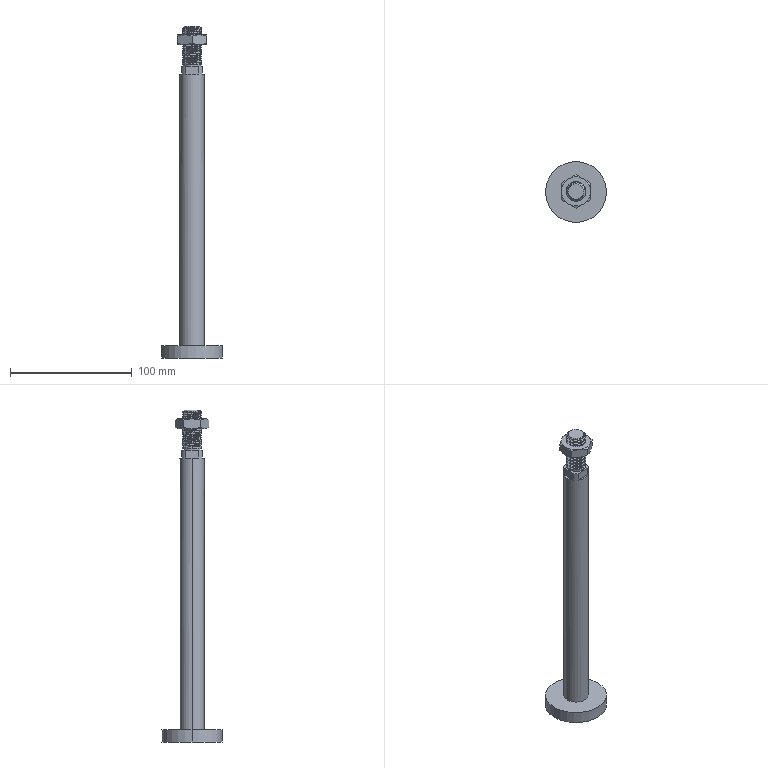Part | SolidWorks | features ICE 5, Revolution 3, RevCut 2, Chamfer 1, Helix 1, LPattern 1, MirrorPattern 1, SweepCut 1 | 1 solid | 78 faces | box 50 x 50 x 272.5 mm | volume 99856 mm3 | cylinder 37 | plane 23 | cone 14 | spline 4 | commonest cylinder face diameters 16 x31 14 x2 20 x2 50 x2